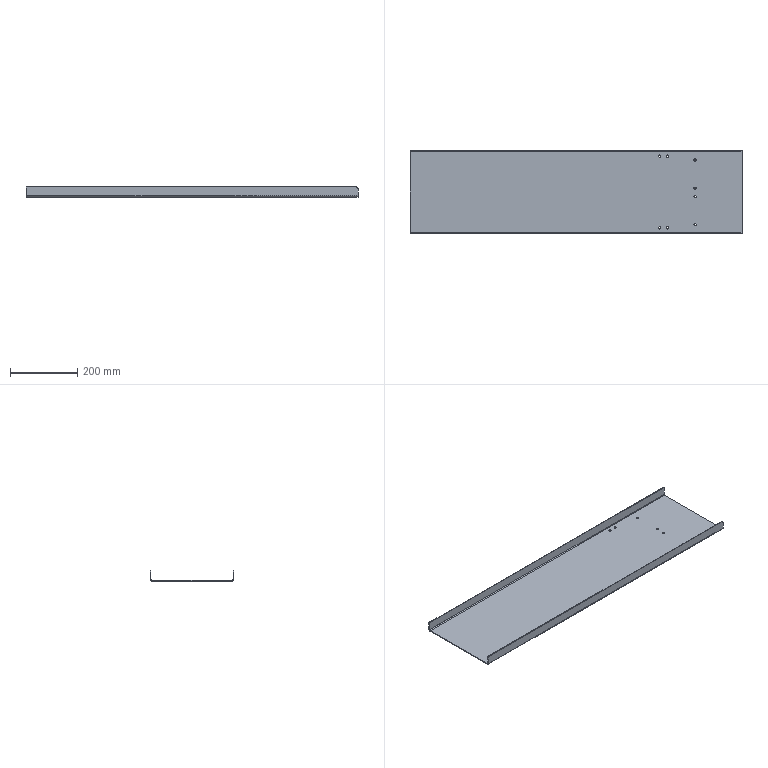Part | STEP file | [01]-8 | 1 solid | 32 faces | box 990 x 250 x 30 mm | volume 687960 mm3 | cylinder 22 | plane 10 | commonest cylinder face diameters 6.8 x16 4.6 x2 9.2 x2 10 x2